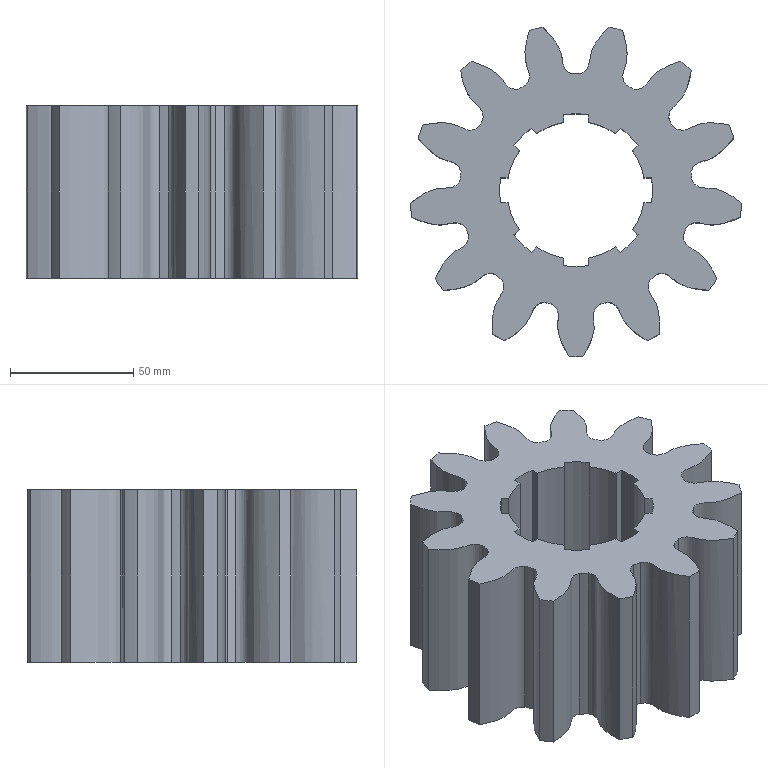Part | SolidWorks | features ICE 2, CirPattern 1, Extrusion 1, RefAxis 1 | 1 solid | 87 faces | box 134.581 x 133.659 x 70 mm | volume 542357 mm3 | cylinder 43 | spline 26 | plane 18 | commonest cylinder face diameters 94.5 x13 135 x13 62 x9 56 x8